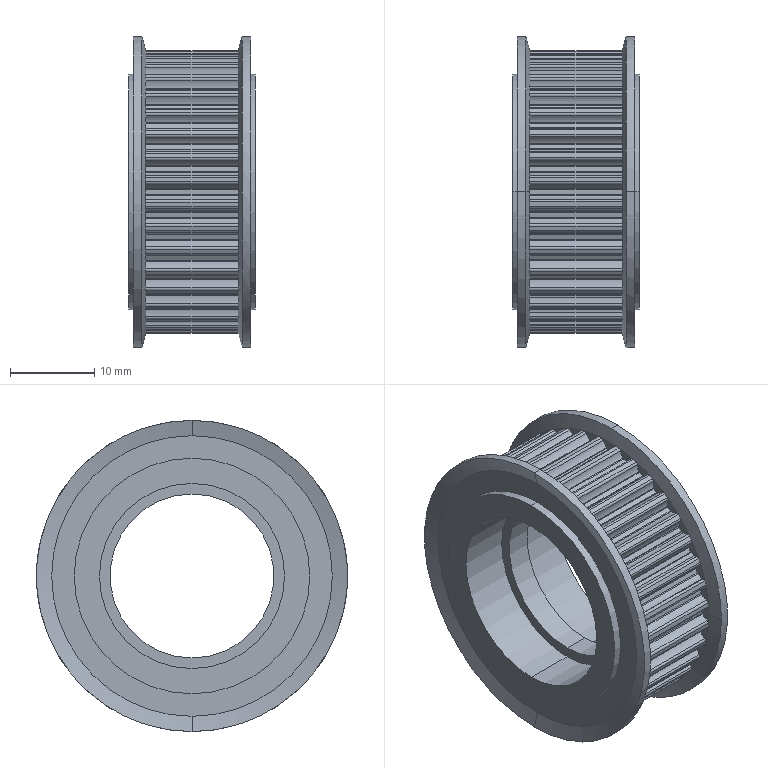Part | STEP file | 11-X_AHTFW36-S3M100-10-FC37_b11 | 1 solid | 421 faces | box 15 x 37 x 37 mm | volume 7051 mm3 | cylinder 335 | plane 78 | cone 8 | commonest cylinder face diameters 0.56 x88 0.3 x82 3.95 x78 31.4 x37 33.62 x36 22 x4